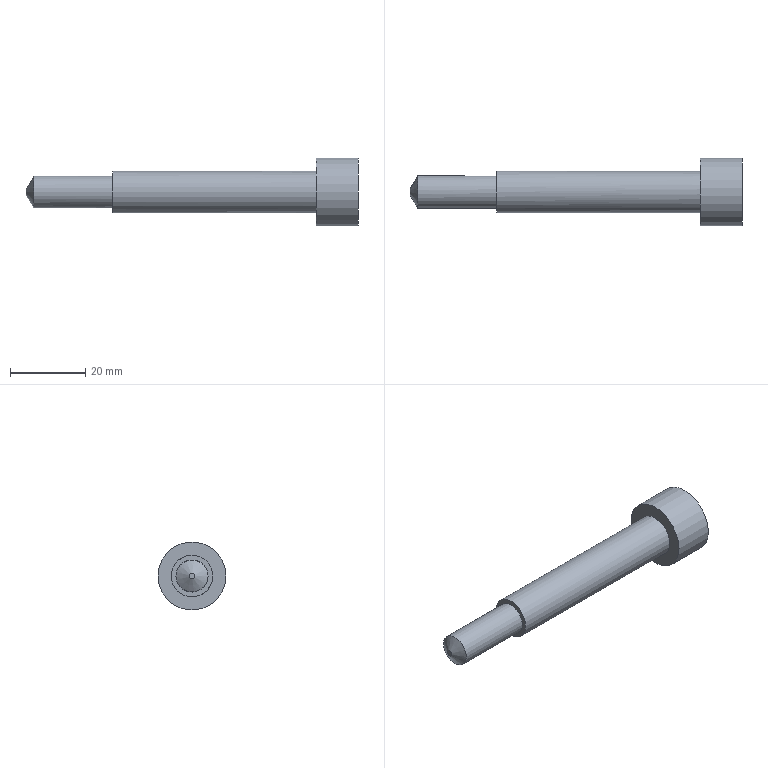Part | STEP file | solid 200 | 1 solid | 8 faces | box 88 x 18 x 18 mm | volume 9169 mm3 | plane 4 | cylinder 3 | cone 1 | commonest cylinder face diameters 8.5 x1 11 x1 18 x1